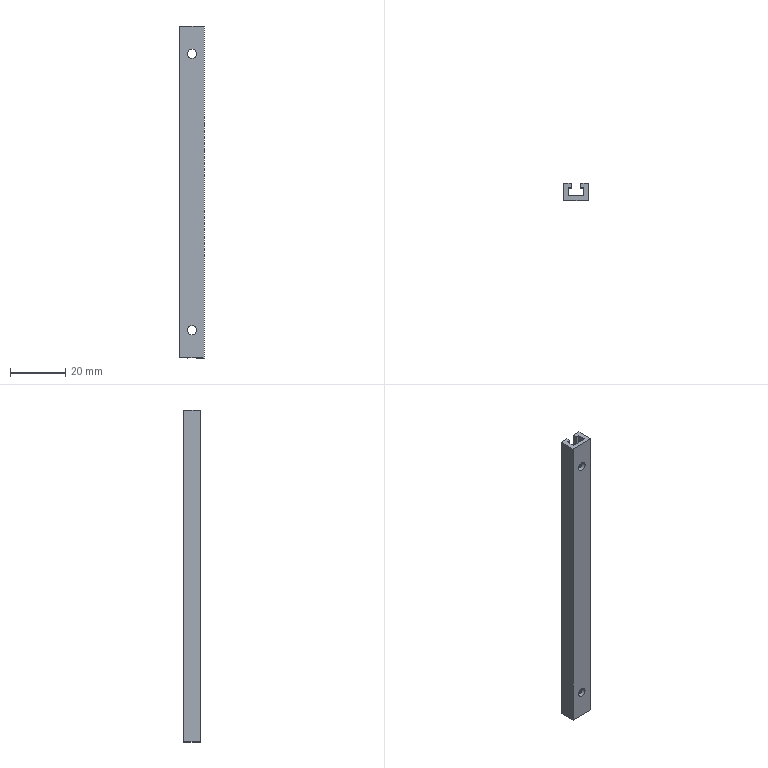Part | NX | 1 solid | 32 faces | box 9 x 6 x 120 mm | volume 3761 mm3 | plane 26 | cylinder 6 | commonest cylinder face diameters 6 x4 3.3 x2
STEP:
#1=CARTESIAN_POINT('',(6.2,-1.5,120.));
#2=VERTEX_POINT('',#1);
#3=CARTESIAN_POINT('',(6.2,-1.5,112.472));
#4=VERTEX_POINT('',#3);
#5=CARTESIAN_POINT('',(6.2,-1.5,120.));
#6=DIRECTION('',(0.,0.,-1.));
#7=VECTOR('',#6,1000.);
#8=LINE('',#5,#7);
#9=EDGE_CURVE('',#2,#4,#8,.T.);
#10=ORIENTED_EDGE('',*,*,#9,.T.);
#11=CARTESIAN_POINT('',(7.35,-1.5,110.937));
#12=VERTEX_POINT('',#11);
#13=CARTESIAN_POINT('',(4.5,-1.5,110.));
#14=DIRECTION('',(0.,1.,0.));
#15=DIRECTION('',(0.,0.,1.));
#16=AXIS2_PLACEMENT_3D('',#13,#14,#15);
#17=CIRCLE('',#16,3.);
#18=EDGE_CURVE('',#4,#12,#17,.T.);
#19=ORIENTED_EDGE('',*,*,#18,.T.);
#20=CARTESIAN_POINT('',(7.35,-1.5,120.));
#21=VERTEX_POINT('',#20);
#22=CARTESIAN_POINT('',(7.35,-1.5,120.));
#23=DIRECTION('',(0.,0.,-1.));
#24=VECTOR('',#23,1000.);
#25=LINE('',#22,#24);
#26=EDGE_CURVE('',#21,#12,#25,.T.);
#27=ORIENTED_EDGE('',*,*,#26,.F.);
#28=CARTESIAN_POINT('',(6.2,-1.5,120.));
#29=DIRECTION('',(1.,0.,0.));
#30=VECTOR('',#29,1000.);
#31=LINE('',#28,#30);
#32=EDGE_CURVE('',#2,#21,#31,.T.);
#33=ORIENTED_EDGE('',*,*,#32,.F.);
#34=EDGE_LOOP('',(#10,#19,#27,#33));
#35=FACE_BOUND('',#34,.T.);
#36=CARTESIAN_POINT('',(6.2,-1.5,120.));
#37=DIRECTION('',(0.,1.,0.));
#38=DIRECTION('',(0.,0.,1.));
#39=AXIS2_PLACEMENT_3D('',#36,#37,#38);
#40=PLANE('',#39);
#41=ADVANCED_FACE('',(#35),#40,.F.);
#42=CARTESIAN_POINT('',(1.65,-4.5,120.));
#43=VERTEX_POINT('',#42);
#44=CARTESIAN_POINT('',(1.65,-4.5,110.937));
#45=VERTEX_POINT('',#44);
#46=CARTESIAN_POINT('',(1.65,-4.5,120.));
#47=DIRECTION('',(0.,0.,-1.));
#48=VECTOR('',#47,1000.);
#49=LINE('',#46,#48);
#50=EDGE_CURVE('',#43,#45,#49,.T.);
#51=ORIENTED_EDGE('',*,*,#50,.T.);
#52=CARTESIAN_POINT('',(1.65,-1.5,110.937));
#53=VERTEX_POINT('',#52);
#54=CARTESIAN_POINT('',(1.65,-4.5,110.937));
#55=DIRECTION('',(0.,1.,0.));
#56=VECTOR('',#55,1000.);
#57=LINE('',#54,#56);
#58=EDGE_CURVE('',#45,#53,#57,.T.);
#59=ORIENTED_EDGE('',*,*,#58,.T.);
#60=CARTESIAN_POINT('',(1.65,-1.5,120.));
#61=VERTEX_POINT('',#60);
#62=CARTESIAN_POINT('',(1.65,-1.5,120.));
#63=DIRECTION('',(0.,0.,-1.));
#64=VECTOR('',#63,1000.);
#65=LINE('',#62,#64);
#66=EDGE_CURVE('',#61,#53,#65,.T.);
#67=ORIENTED_EDGE('',*,*,#66,.F.);
#68=CARTESIAN_POINT('',(1.65,-4.5,120.));
#69=DIRECTION('',(0.,1.,0.));
#70=VECTOR('',#69,1000.);
#71=LINE('',#68,#70);
#72=EDGE_CURVE('',#43,#61,#71,.T.);
#73=ORIENTED_EDGE('',*,*,#72,.F.);
#74=EDGE_LOOP('',(#51,#59,#67,#73));
#75=FACE_BOUND('',#74,.T.);
#76=CARTESIAN_POINT('',(1.65,-4.5,120.));
#77=DIRECTION('',(-1.,0.,0.));
#78=DIRECTION('',(0.,0.,1.));
#79=AXIS2_PLACEMENT_3D('',#76,#77,#78);
#80=PLANE('',#79);
#81=ADVANCED_FACE('',(#75),#80,.F.);
#82=CARTESIAN_POINT('',(2.8,-1.5,120.));
#83=VERTEX_POINT('',#82);
#84=CARTESIAN_POINT('',(2.8,-1.5,112.472));
#85=VERTEX_POINT('',#84);
#86=CARTESIAN_POINT('',(2.8,-1.5,120.));
#87=DIRECTION('',(0.,0.,-1.));
#88=VECTOR('',#87,1000.);
#89=LINE('',#86,#88);
#90=EDGE_CURVE('',#83,#85,#89,.T.);
#91=ORIENTED_EDGE('',*,*,#90,.T.);
#92=CARTESIAN_POINT('',(2.8,0.,112.472));
#93=VERTEX_POINT('',#92);
#94=CARTESIAN_POINT('',(2.8,-4.5,112.472));
#95=DIRECTION('',(0.,1.,0.));
#96=VECTOR('',#95,1000.);
#97=LINE('',#94,#96);
#98=EDGE_CURVE('',#85,#93,#97,.T.);
#99=ORIENTED_EDGE('',*,*,#98,.T.);
#100=CARTESIAN_POINT('',(2.8,0.,120.));
#101=VERTEX_POINT('',#100);
#102=CARTESIAN_POINT('',(2.8,0.,120.));
#103=DIRECTION('',(0.,0.,-1.));
#104=VECTOR('',#103,1000.);
#105=LINE('',#102,#104);
#106=EDGE_CURVE('',#101,#93,#105,.T.);
#107=ORIENTED_EDGE('',*,*,#106,.F.);
#108=CARTESIAN_POINT('',(2.8,-1.5,120.));
#109=DIRECTION('',(0.,1.,0.));
#110=VECTOR('',#109,1000.);
#111=LINE('',#108,#110);
#112=EDGE_CURVE('',#83,#101,#111,.T.);
#113=ORIENTED_EDGE('',*,*,#112,.F.);
#114=EDGE_LOOP('',(#91,#99,#107,#113));
#115=FACE_BOUND('',#114,.T.);
#116=CARTESIAN_POINT('',(2.8,-1.5,120.));
#117=DIRECTION('',(-1.,0.,0.));
#118=DIRECTION('',(0.,0.,1.));
#119=AXIS2_PLACEMENT_3D('',#116,#117,#118);
#120=PLANE('',#119);
#121=ADVANCED_FACE('',(#115),#120,.F.);
#122=CARTESIAN_POINT('',(6.2,-1.5,107.528));
#123=VERTEX_POINT('',#122);
#124=CARTESIAN_POINT('',(6.2,-1.5,12.472));
#125=VERTEX_POINT('',#124);
#126=CARTESIAN_POINT('',(6.2,-1.5,120.));
#127=DIRECTION('',(0.,0.,-1.));
#128=VECTOR('',#127,1000.);
#129=LINE('',#126,#128);
#130=EDGE_CURVE('',#123,#125,#129,.T.);
#131=ORIENTED_EDGE('',*,*,#130,.F.);
#132=CARTESIAN_POINT('',(6.2,0.,107.528));
#133=VERTEX_POINT('',#132);
#134=CARTESIAN_POINT('',(6.2,-4.5,107.528));
#135=DIRECTION('',(0.,1.,0.));
#136=VECTOR('',#135,1000.);
#137=LINE('',#134,#136);
#138=EDGE_CURVE('',#123,#133,#137,.T.);
#139=ORIENTED_EDGE('',*,*,#138,.T.);
#140=CARTESIAN_POINT('',(6.2,0.,12.472));
#141=VERTEX_POINT('',#140);
#142=CARTESIAN_POINT('',(6.2,0.,120.));
#143=DIRECTION('',(0.,0.,-1.));
#144=VECTOR('',#143,1000.);
#145=LINE('',#142,#144);
#146=EDGE_CURVE('',#133,#141,#145,.T.);
#147=ORIENTED_EDGE('',*,*,#146,.T.);
#148=CARTESIAN_POINT('',(6.2,-4.5,12.472));
#149=DIRECTION('',(0.,1.,0.));
#150=VECTOR('',#149,1000.);
#151=LINE('',#148,#150);
#152=EDGE_CURVE('',#141,#125,#151,.F.);
#153=ORIENTED_EDGE('',*,*,#152,.T.);
#154=EDGE_LOOP('',(#131,#139,#147,#153));
#155=FACE_BOUND('',#154,.T.);
#156=CARTESIAN_POINT('',(6.2,0.,120.));
#157=DIRECTION('',(1.,0.,0.));
#158=DIRECTION('',(0.,0.,-1.));
#159=AXIS2_PLACEMENT_3D('',#156,#157,#158);
#160=PLANE('',#159);
#161=ADVANCED_FACE('',(#155),#160,.F.);
#162=CARTESIAN_POINT('',(7.35,-4.5,109.063));
#163=VERTEX_POINT('',#162);
#164=CARTESIAN_POINT('',(7.35,-4.5,10.937));
#165=VERTEX_POINT('',#164);
#166=CARTESIAN_POINT('',(7.35,-4.5,120.));
#167=DIRECTION('',(0.,0.,-1.));
#168=VECTOR('',#167,1000.);
#169=LINE('',#166,#168);
#170=EDGE_CURVE('',#163,#165,#169,.T.);
#171=ORIENTED_EDGE('',*,*,#170,.F.);
#172=CARTESIAN_POINT('',(7.35,-1.5,109.063));
#173=VERTEX_POINT('',#172);
#174=CARTESIAN_POINT('',(7.35,-4.5,109.063));
#175=DIRECTION('',(0.,1.,0.));
#176=VECTOR('',#175,1000.);
#177=LINE('',#174,#176);
#178=EDGE_CURVE('',#163,#173,#177,.T.);
#179=ORIENTED_EDGE('',*,*,#178,.T.);
#180=CARTESIAN_POINT('',(7.35,-1.5,10.937));
#181=VERTEX_POINT('',#180);
#182=CARTESIAN_POINT('',(7.35,-1.5,120.));
#183=DIRECTION('',(0.,0.,-1.));
#184=VECTOR('',#183,1000.);
#185=LINE('',#182,#184);
#186=EDGE_CURVE('',#173,#181,#185,.T.);
#187=ORIENTED_EDGE('',*,*,#186,.T.);
#188=CARTESIAN_POINT('',(7.35,-4.5,10.937));
#189=DIRECTION('',(0.,1.,0.));
#190=VECTOR('',#189,1000.);
#191=LINE('',#188,#190);
#192=EDGE_CURVE('',#181,#165,#191,.F.);
#193=ORIENTED_EDGE('',*,*,#192,.T.);
#194=EDGE_LOOP('',(#171,#179,#187,#193));
#195=FACE_BOUND('',#194,.T.);
#196=CARTESIAN_POINT('',(7.35,-1.5,120.));
#197=DIRECTION('',(1.,0.,0.));
#198=DIRECTION('',(0.,0.,-1.));
#199=AXIS2_PLACEMENT_3D('',#196,#197,#198);
#200=PLANE('',#199);
#201=ADVANCED_FACE('',(#195),#200,.F.);
#202=CARTESIAN_POINT('',(2.8,-1.5,107.528));
#203=VERTEX_POINT('',#202);
#204=CARTESIAN_POINT('',(2.8,-1.5,12.472));
#205=VERTEX_POINT('',#204);
#206=CARTESIAN_POINT('',(2.8,-1.5,120.));
#207=DIRECTION('',(0.,0.,-1.));
#208=VECTOR('',#207,1000.);
#209=LINE('',#206,#208);
#210=EDGE_CURVE('',#203,#205,#209,.T.);
#211=ORIENTED_EDGE('',*,*,#210,.F.);
#212=CARTESIAN_POINT('',(1.65,-1.5,109.063));
#213=VERTEX_POINT('',#212);
#214=CARTESIAN_POINT('',(4.5,-1.5,110.));
#215=DIRECTION('',(0.,1.,0.));
#216=DIRECTION('',(0.,0.,1.));
#217=AXIS2_PLACEMENT_3D('',#214,#215,#216);
#218=CIRCLE('',#217,3.);
#219=EDGE_CURVE('',#203,#213,#218,.T.);
#220=ORIENTED_EDGE('',*,*,#219,.T.);
#221=CARTESIAN_POINT('',(1.65,-1.5,10.937));
#222=VERTEX_POINT('',#221);
#223=CARTESIAN_POINT('',(1.65,-1.5,120.));
#224=DIRECTION('',(0.,0.,-1.));
#225=VECTOR('',#224,1000.);
#226=LINE('',#223,#225);
#227=EDGE_CURVE('',#213,#222,#226,.T.);
#228=ORIENTED_EDGE('',*,*,#227,.T.);
#229=CARTESIAN_POINT('',(4.5,-1.5,10.));
#230=DIRECTION('',(0.,1.,0.));
#231=DIRECTION('',(0.,0.,1.));
#232=AXIS2_PLACEMENT_3D('',#229,#230,#231);
#233=CIRCLE('',#232,3.);
#234=EDGE_CURVE('',#222,#205,#233,.T.);
#235=ORIENTED_EDGE('',*,*,#234,.T.);
#236=EDGE_LOOP('',(#211,#220,#228,#235));
#237=FACE_BOUND('',#236,.T.);
#238=CARTESIAN_POINT('',(1.65,-1.5,120.));
#239=DIRECTION('',(0.,1.,0.));
#240=DIRECTION('',(0.,0.,1.));
#241=AXIS2_PLACEMENT_3D('',#238,#239,#240);
#242=PLANE('',#241);
#243=ADVANCED_FACE('',(#237),#242,.F.);
#244=CARTESIAN_POINT('',(6.2,-1.5,7.528));
#245=VERTEX_POINT('',#244);
#246=CARTESIAN_POINT('',(6.2,-1.5,0.));
#247=VERTEX_POINT('',#246);
#248=CARTESIAN_POINT('',(6.2,-1.5,120.));
#249=DIRECTION('',(0.,0.,-1.));
#250=VECTOR('',#249,1000.);
#251=LINE('',#248,#250);
#252=EDGE_CURVE('',#245,#247,#251,.T.);
#253=ORIENTED_EDGE('',*,*,#252,.F.);
#254=CARTESIAN_POINT('',(6.2,0.,7.528));
#255=VERTEX_POINT('',#254);
#256=CARTESIAN_POINT('',(6.2,-4.5,7.528));
#257=DIRECTION('',(0.,1.,0.));
#258=VECTOR('',#257,1000.);
#259=LINE('',#256,#258);
#260=EDGE_CURVE('',#245,#255,#259,.T.);
#261=ORIENTED_EDGE('',*,*,#260,.T.);
#262=CARTESIAN_POINT('',(6.2,0.,0.));
#263=VERTEX_POINT('',#262);
#264=CARTESIAN_POINT('',(6.2,0.,120.));
#265=DIRECTION('',(0.,0.,-1.));
#266=VECTOR('',#265,1000.);
#267=LINE('',#264,#266);
#268=EDGE_CURVE('',#255,#263,#267,.T.);
#269=ORIENTED_EDGE('',*,*,#268,.T.);
#270=CARTESIAN_POINT('',(6.2,0.,0.));
#271=DIRECTION('',(0.,-1.,0.));
#272=VECTOR('',#271,1000.);
#273=LINE('',#270,#272);
#274=EDGE_CURVE('',#263,#247,#273,.T.);
#275=ORIENTED_EDGE('',*,*,#274,.T.);
#276=EDGE_LOOP('',(#253,#261,#269,#275));
#277=FACE_BOUND('',#276,.T.);
#278=CARTESIAN_POINT('',(6.2,0.,120.));
#279=DIRECTION('',(1.,0.,0.));
#280=DIRECTION('',(0.,0.,-1.));
#281=AXIS2_PLACEMENT_3D('',#278,#279,#280);
#282=PLANE('',#281);
#283=ADVANCED_FACE('',(#277),#282,.F.);
#284=ORIENTED_EDGE('',*,*,#186,.F.);
#285=CARTESIAN_POINT('',(4.5,-1.5,110.));
#286=DIRECTION('',(0.,1.,0.));
#287=DIRECTION('',(0.,0.,1.));
#288=AXIS2_PLACEMENT_3D('',#285,#286,#287);
#289=CIRCLE('',#288,3.);
#290=EDGE_CURVE('',#173,#123,#289,.T.);
#291=ORIENTED_EDGE('',*,*,#290,.T.);
#292=ORIENTED_EDGE('',*,*,#130,.T.);
#293=CARTESIAN_POINT('',(4.5,-1.5,10.));
#294=DIRECTION('',(0.,1.,0.));
#295=DIRECTION('',(0.,0.,1.));
#296=AXIS2_PLACEMENT_3D('',#293,#294,#295);
#297=CIRCLE('',#296,3.);
#298=EDGE_CURVE('',#125,#181,#297,.T.);
#299=ORIENTED_EDGE('',*,*,#298,.T.);
#300=EDGE_LOOP('',(#284,#291,#292,#299));
#301=FACE_BOUND('',#300,.T.);
#302=CARTESIAN_POINT('',(6.2,-1.5,120.));
#303=DIRECTION('',(0.,1.,0.));
#304=DIRECTION('',(0.,0.,1.));
#305=AXIS2_PLACEMENT_3D('',#302,#303,#304);
#306=PLANE('',#305);
#307=ADVANCED_FACE('',(#301),#306,.F.);
#308=CARTESIAN_POINT('',(7.35,-4.5,9.063));
#309=VERTEX_POINT('',#308);
#310=CARTESIAN_POINT('',(7.35,-4.5,0.));
#311=VERTEX_POINT('',#310);
#312=CARTESIAN_POINT('',(7.35,-4.5,120.));
#313=DIRECTION('',(0.,0.,-1.));
#314=VECTOR('',#313,1000.);
#315=LINE('',#312,#314);
#316=EDGE_CURVE('',#309,#311,#315,.T.);
#317=ORIENTED_EDGE('',*,*,#316,.F.);
#318=CARTESIAN_POINT('',(7.35,-1.5,9.063));
#319=VERTEX_POINT('',#318);
#320=CARTESIAN_POINT('',(7.35,-4.5,9.063));
#321=DIRECTION('',(0.,1.,0.));
#322=VECTOR('',#321,1000.);
#323=LINE('',#320,#322);
#324=EDGE_CURVE('',#309,#319,#323,.T.);
#325=ORIENTED_EDGE('',*,*,#324,.T.);
#326=CARTESIAN_POINT('',(7.35,-1.5,0.));
#327=VERTEX_POINT('',#326);
#328=CARTESIAN_POINT('',(7.35,-1.5,120.));
#329=DIRECTION('',(0.,0.,-1.));
#330=VECTOR('',#329,1000.);
#331=LINE('',#328,#330);
#332=EDGE_CURVE('',#319,#327,#331,.T.);
#333=ORIENTED_EDGE('',*,*,#332,.T.);
#334=CARTESIAN_POINT('',(7.35,-1.5,0.));
#335=DIRECTION('',(0.,-1.,0.));
#336=VECTOR('',#335,1000.);
#337=LINE('',#334,#336);
#338=EDGE_CURVE('',#327,#311,#337,.T.);
#339=ORIENTED_EDGE('',*,*,#338,.T.);
#340=EDGE_LOOP('',(#317,#325,#333,#339));
#341=FACE_BOUND('',#340,.T.);
#342=CARTESIAN_POINT('',(7.35,-1.5,120.));
#343=DIRECTION('',(1.,0.,0.));
#344=DIRECTION('',(0.,0.,-1.));
#345=AXIS2_PLACEMENT_3D('',#342,#343,#344);
#346=PLANE('',#345);
#347=ADVANCED_FACE('',(#341),#346,.F.);
#348=ORIENTED_EDGE('',*,*,#227,.F.);
#349=CARTESIAN_POINT('',(1.65,-4.5,109.063));
#350=VERTEX_POINT('',#349);
#351=CARTESIAN_POINT('',(1.65,-4.5,109.063));
#352=DIRECTION('',(0.,1.,0.));
#353=VECTOR('',#352,1000.);
#354=LINE('',#351,#353);
#355=EDGE_CURVE('',#213,#350,#354,.F.);
#356=ORIENTED_EDGE('',*,*,#355,.T.);
#357=CARTESIAN_POINT('',(1.65,-4.5,10.937));
#358=VERTEX_POINT('',#357);
#359=CARTESIAN_POINT('',(1.65,-4.5,120.));
#360=DIRECTION('',(0.,0.,-1.));
#361=VECTOR('',#360,1000.);
#362=LINE('',#359,#361);
#363=EDGE_CURVE('',#350,#358,#362,.T.);
#364=ORIENTED_EDGE('',*,*,#363,.T.);
#365=CARTESIAN_POINT('',(1.65,-4.5,10.937));
#366=DIRECTION('',(0.,1.,0.));
#367=VECTOR('',#366,1000.);
#368=LINE('',#365,#367);
#369=EDGE_CURVE('',#358,#222,#368,.T.);
#370=ORIENTED_EDGE('',*,*,#369,.T.);
#371=EDGE_LOOP('',(#348,#356,#364,#370));
#372=FACE_BOUND('',#371,.T.);
#373=CARTESIAN_POINT('',(1.65,-4.5,120.));
#374=DIRECTION('',(-1.,0.,0.));
#375=DIRECTION('',(0.,0.,1.));
#376=AXIS2_PLACEMENT_3D('',#373,#374,#375);
#377=PLANE('',#376);
#378=ADVANCED_FACE('',(#372),#377,.F.);
#379=CARTESIAN_POINT('',(2.8,-1.5,7.528));
#380=VERTEX_POINT('',#379);
#381=CARTESIAN_POINT('',(2.8,-1.5,0.));
#382=VERTEX_POINT('',#381);
#383=CARTESIAN_POINT('',(2.8,-1.5,120.));
#384=DIRECTION('',(0.,0.,-1.));
#385=VECTOR('',#384,1000.);
#386=LINE('',#383,#385);
#387=EDGE_CURVE('',#380,#382,#386,.T.);
#388=ORIENTED_EDGE('',*,*,#387,.F.);
#389=CARTESIAN_POINT('',(1.65,-1.5,9.063));
#390=VERTEX_POINT('',#389);
#391=CARTESIAN_POINT('',(4.5,-1.5,10.));
#392=DIRECTION('',(0.,1.,0.));
#393=DIRECTION('',(0.,0.,1.));
#394=AXIS2_PLACEMENT_3D('',#391,#392,#393);
#395=CIRCLE('',#394,3.);
#396=EDGE_CURVE('',#380,#390,#395,.T.);
#397=ORIENTED_EDGE('',*,*,#396,.T.);
#398=CARTESIAN_POINT('',(1.65,-1.5,0.));
#399=VERTEX_POINT('',#398);
#400=CARTESIAN_POINT('',(1.65,-1.5,120.));
#401=DIRECTION('',(0.,0.,-1.));
#402=VECTOR('',#401,1000.);
#403=LINE('',#400,#402);
#404=EDGE_CURVE('',#390,#399,#403,.T.);
#405=ORIENTED_EDGE('',*,*,#404,.T.);
#406=CARTESIAN_POINT('',(1.65,-1.5,0.));
#407=DIRECTION('',(1.,0.,0.));
#408=VECTOR('',#407,1000.);
#409=LINE('',#406,#408);
#410=EDGE_CURVE('',#399,#382,#409,.T.);
#411=ORIENTED_EDGE('',*,*,#410,.T.);
#412=EDGE_LOOP('',(#388,#397,#405,#411));
#413=FACE_BOUND('',#412,.T.);
#414=CARTESIAN_POINT('',(1.65,-1.5,120.));
#415=DIRECTION('',(0.,1.,0.));
#416=DIRECTION('',(0.,0.,1.));
#417=AXIS2_PLACEMENT_3D('',#414,#415,#416);
#418=PLANE('',#417);
#419=ADVANCED_FACE('',(#413),#418,.F.);
#420=CARTESIAN_POINT('',(2.8,0.,107.528));
#421=VERTEX_POINT('',#420);
#422=CARTESIAN_POINT('',(2.8,0.,12.472));
#423=VERTEX_POINT('',#422);
#424=CARTESIAN_POINT('',(2.8,0.,120.));
#425=DIRECTION('',(0.,0.,-1.));
#426=VECTOR('',#425,1000.);
#427=LINE('',#424,#426);
#428=EDGE_CURVE('',#421,#423,#427,.T.);
#429=ORIENTED_EDGE('',*,*,#428,.F.);
#430=CARTESIAN_POINT('',(2.8,-4.5,107.528));
#431=DIRECTION('',(0.,1.,0.));
#432=VECTOR('',#431,1000.);
#433=LINE('',#430,#432);
#434=EDGE_CURVE('',#421,#203,#433,.F.);
#435=ORIENTED_EDGE('',*,*,#434,.T.);
#436=ORIENTED_EDGE('',*,*,#210,.T.);
#437=CARTESIAN_POINT('',(2.8,-4.5,12.472));
#438=DIRECTION('',(0.,1.,0.));
#439=VECTOR('',#438,1000.);
#440=LINE('',#437,#439);
#441=EDGE_CURVE('',#205,#423,#440,.T.);
#442=ORIENTED_EDGE('',*,*,#441,.T.);
#443=EDGE_LOOP('',(#429,#435,#436,#442));
#444=FACE_BOUND('',#443,.T.);
#445=CARTESIAN_POINT('',(2.8,-1.5,120.));
#446=DIRECTION('',(-1.,0.,0.));
#447=DIRECTION('',(0.,0.,1.));
#448=AXIS2_PLACEMENT_3D('',#445,#446,#447);
#449=PLANE('',#448);
#450=ADVANCED_FACE('',(#444),#449,.F.);
#451=ORIENTED_EDGE('',*,*,#106,.T.);
#452=CARTESIAN_POINT('',(4.5,0.,110.));
#453=DIRECTION('',(0.,1.,0.));
#454=DIRECTION('',(-1.,0.,0.));
#455=AXIS2_PLACEMENT_3D('',#452,#453,#454);
#456=CIRCLE('',#455,3.);
#457=EDGE_CURVE('',#421,#93,#456,.T.);
#458=ORIENTED_EDGE('',*,*,#457,.F.);
#459=ORIENTED_EDGE('',*,*,#428,.T.);
#460=CARTESIAN_POINT('',(2.8,0.,7.528));
#461=VERTEX_POINT('',#460);
#462=CARTESIAN_POINT('',(4.5,0.,10.));
#463=DIRECTION('',(0.,1.,0.));
#464=DIRECTION('',(-1.,0.,0.));
#465=AXIS2_PLACEMENT_3D('',#462,#463,#464);
#466=CIRCLE('',#465,3.);
#467=EDGE_CURVE('',#461,#423,#466,.T.);
#468=ORIENTED_EDGE('',*,*,#467,.F.);
#469=CARTESIAN_POINT('',(2.8,0.,0.));
#470=VERTEX_POINT('',#469);
#471=CARTESIAN_POINT('',(2.8,0.,120.));
#472=DIRECTION('',(0.,0.,-1.));
#473=VECTOR('',#472,1000.);
#474=LINE('',#471,#473);
#475=EDGE_CURVE('',#461,#470,#474,.T.);
#476=ORIENTED_EDGE('',*,*,#475,.T.);
#477=CARTESIAN_POINT('',(0.,0.,0.));
#478=VERTEX_POINT('',#477);
#479=CARTESIAN_POINT('',(2.8,0.,0.));
#480=DIRECTION('',(-1.,0.,0.));
#481=VECTOR('',#480,1000.);
#482=LINE('',#479,#481);
#483=EDGE_CURVE('',#470,#478,#482,.T.);
#484=ORIENTED_EDGE('',*,*,#483,.T.);
#485=CARTESIAN_POINT('',(0.,0.,120.));
#486=VERTEX_POINT('',#485);
#487=CARTESIAN_POINT('',(0.,0.,120.));
#488=DIRECTION('',(0.,0.,-1.));
#489=VECTOR('',#488,1000.);
#490=LINE('',#487,#489);
#491=EDGE_CURVE('',#486,#478,#490,.T.);
#492=ORIENTED_EDGE('',*,*,#491,.F.);
#493=CARTESIAN_POINT('',(2.8,0.,120.));
#494=DIRECTION('',(-1.,0.,0.));
#495=VECTOR('',#494,1000.);
#496=LINE('',#493,#495);
#497=EDGE_CURVE('',#101,#486,#496,.T.);
#498=ORIENTED_EDGE('',*,*,#497,.F.);
#499=EDGE_LOOP('',(#451,#458,#459,#468,#476,#484,#492,#498));
#500=FACE_BOUND('',#499,.T.);
#501=CARTESIAN_POINT('',(2.8,0.,120.));
#502=DIRECTION('',(0.,-1.,0.));
#503=DIRECTION('',(1.,0.,0.));
#504=AXIS2_PLACEMENT_3D('',#501,#502,#503);
#505=PLANE('',#504);
#506=ADVANCED_FACE('',(#500),#505,.F.);
#507=CARTESIAN_POINT('',(0.,-6.,0.));
#508=VERTEX_POINT('',#507);
#509=CARTESIAN_POINT('',(0.,0.,0.));
#510=DIRECTION('',(0.,-1.,0.));
#511=VECTOR('',#510,1000.);
#512=LINE('',#509,#511);
#513=EDGE_CURVE('',#478,#508,#512,.T.);
#514=ORIENTED_EDGE('',*,*,#513,.T.);
#515=CARTESIAN_POINT('',(0.,-6.,120.));
#516=VERTEX_POINT('',#515);
#517=CARTESIAN_POINT('',(0.,-6.,120.));
#518=DIRECTION('',(0.,0.,-1.));
#519=VECTOR('',#518,1000.);
#520=LINE('',#517,#519);
#521=EDGE_CURVE('',#516,#508,#520,.T.);
#522=ORIENTED_EDGE('',*,*,#521,.F.);
#523=CARTESIAN_POINT('',(0.,0.,120.));
#524=DIRECTION('',(0.,-1.,0.));
#525=VECTOR('',#524,1000.);
#526=LINE('',#523,#525);
#527=EDGE_CURVE('',#486,#516,#526,.T.);
#528=ORIENTED_EDGE('',*,*,#527,.F.);
#529=ORIENTED_EDGE('',*,*,#491,.T.);
#530=EDGE_LOOP('',(#514,#522,#528,#529));
#531=FACE_BOUND('',#530,.T.);
#532=CARTESIAN_POINT('',(0.,0.,120.));
#533=DIRECTION('',(1.,0.,0.));
#534=DIRECTION('',(0.,1.,0.));
#535=AXIS2_PLACEMENT_3D('',#532,#533,#534);
#536=PLANE('',#535);
#537=ADVANCED_FACE('',(#531),#536,.F.);
#538=CARTESIAN_POINT('',(4.5,-6.,11.65));
#539=VERTEX_POINT('',#538);
#540=CARTESIAN_POINT('',(4.5,-6.,10.));
#541=DIRECTION('',(0.,1.,0.));
#542=DIRECTION('',(0.,0.,1.));
#543=AXIS2_PLACEMENT_3D('',#540,#541,#542);
#544=CIRCLE('',#543,1.65);
#545=EDGE_CURVE('',#539,#539,#544,.T.);
#546=ORIENTED_EDGE('',*,*,#545,.T.);
#547=EDGE_LOOP('',(#546));
#548=FACE_BOUND('',#547,.T.);
#549=CARTESIAN_POINT('',(4.5,-6.,111.65));
#550=VERTEX_POINT('',#549);
#551=CARTESIAN_POINT('',(4.5,-6.,110.));
#552=DIRECTION('',(0.,1.,0.));
#553=DIRECTION('',(0.,0.,1.));
#554=AXIS2_PLACEMENT_3D('',#551,#552,#553);
#555=CIRCLE('',#554,1.65);
#556=EDGE_CURVE('',#550,#550,#555,.T.);
#557=ORIENTED_EDGE('',*,*,#556,.T.);
#558=EDGE_LOOP('',(#557));
#559=FACE_BOUND('',#558,.T.);
#560=CARTESIAN_POINT('',(9.,-6.,0.));
#561=VERTEX_POINT('',#560);
#562=CARTESIAN_POINT('',(0.,-6.,0.));
#563=DIRECTION('',(1.,0.,0.));
#564=VECTOR('',#563,1000.);
#565=LINE('',#562,#564);
#566=EDGE_CURVE('',#508,#561,#565,.T.);
#567=ORIENTED_EDGE('',*,*,#566,.T.);
#568=CARTESIAN_POINT('',(9.,-6.,120.));
#569=VERTEX_POINT('',#568);
#570=CARTESIAN_POINT('',(9.,-6.,120.));
#571=DIRECTION('',(0.,0.,-1.));
#572=VECTOR('',#571,1000.);
#573=LINE('',#570,#572);
#574=EDGE_CURVE('',#569,#561,#573,.T.);
#575=ORIENTED_EDGE('',*,*,#574,.F.);
#576=CARTESIAN_POINT('',(0.,-6.,120.));
#577=DIRECTION('',(1.,0.,0.));
#578=VECTOR('',#577,1000.);
#579=LINE('',#576,#578);
#580=EDGE_CURVE('',#516,#569,#579,.T.);
#581=ORIENTED_EDGE('',*,*,#580,.F.);
#582=ORIENTED_EDGE('',*,*,#521,.T.);
#583=EDGE_LOOP('',(#567,#575,#581,#582));
#584=FACE_BOUND('',#583,.T.);
#585=CARTESIAN_POINT('',(0.,-6.,120.));
#586=DIRECTION('',(0.,1.,0.));
#587=DIRECTION('',(0.,0.,1.));
#588=AXIS2_PLACEMENT_3D('',#585,#586,#587);
#589=PLANE('',#588);
#590=ADVANCED_FACE('',(#548,#559,#584),#589,.F.);
#591=CARTESIAN_POINT('',(9.,0.,0.));
#592=VERTEX_POINT('',#591);
#593=CARTESIAN_POINT('',(9.,-6.,0.));
#594=DIRECTION('',(0.,1.,0.));
#595=VECTOR('',#594,1000.);
#596=LINE('',#593,#595);
#597=EDGE_CURVE('',#561,#592,#596,.T.);
#598=ORIENTED_EDGE('',*,*,#597,.T.);
#599=CARTESIAN_POINT('',(9.,0.,120.));
#600=VERTEX_POINT('',#599);
#601=CARTESIAN_POINT('',(9.,0.,120.));
#602=DIRECTION('',(0.,0.,-1.));
#603=VECTOR('',#602,1000.);
#604=LINE('',#601,#603);
#605=EDGE_CURVE('',#600,#592,#604,.T.);
#606=ORIENTED_EDGE('',*,*,#605,.F.);
#607=CARTESIAN_POINT('',(9.,-6.,120.));
#608=DIRECTION('',(0.,1.,0.));
#609=VECTOR('',#608,1000.);
#610=LINE('',#607,#609);
#611=EDGE_CURVE('',#569,#600,#610,.T.);
#612=ORIENTED_EDGE('',*,*,#611,.F.);
#613=ORIENTED_EDGE('',*,*,#574,.T.);
#614=EDGE_LOOP('',(#598,#606,#612,#613));
#615=FACE_BOUND('',#614,.T.);
#616=CARTESIAN_POINT('',(9.,-6.,120.));
#617=DIRECTION('',(-1.,0.,0.));
#618=DIRECTION('',(0.,0.,1.));
#619=AXIS2_PLACEMENT_3D('',#616,#617,#618);
#620=PLANE('',#619);
#621=ADVANCED_FACE('',(#615),#620,.F.);
#622=ORIENTED_EDGE('',*,*,#146,.F.);
#623=CARTESIAN_POINT('',(6.2,0.,112.472));
#624=VERTEX_POINT('',#623);
#625=CARTESIAN_POINT('',(4.5,0.,110.));
#626=DIRECTION('',(0.,1.,0.));
#627=DIRECTION('',(-1.,0.,0.));
#628=AXIS2_PLACEMENT_3D('',#625,#626,#627);
#629=CIRCLE('',#628,3.);
#630=EDGE_CURVE('',#624,#133,#629,.T.);
#631=ORIENTED_EDGE('',*,*,#630,.F.);
#632=CARTESIAN_POINT('',(6.2,0.,120.));
#633=VERTEX_POINT('',#632);
#634=CARTESIAN_POINT('',(6.2,0.,120.));
#635=DIRECTION('',(0.,0.,-1.));
#636=VECTOR('',#635,1000.);
#637=LINE('',#634,#636);
#638=EDGE_CURVE('',#633,#624,#637,.T.);
#639=ORIENTED_EDGE('',*,*,#638,.F.);
#640=CARTESIAN_POINT('',(9.,0.,120.));
#641=DIRECTION('',(-1.,0.,0.));
#642=VECTOR('',#641,1000.);
#643=LINE('',#640,#642);
#644=EDGE_CURVE('',#600,#633,#643,.T.);
#645=ORIENTED_EDGE('',*,*,#644,.F.);
#646=ORIENTED_EDGE('',*,*,#605,.T.);
#647=CARTESIAN_POINT('',(9.,0.,0.));
#648=DIRECTION('',(-1.,0.,0.));
#649=VECTOR('',#648,1000.);
#650=LINE('',#647,#649);
#651=EDGE_CURVE('',#592,#263,#650,.T.);
#652=ORIENTED_EDGE('',*,*,#651,.T.);
#653=ORIENTED_EDGE('',*,*,#268,.F.);
#654=CARTESIAN_POINT('',(4.5,0.,10.));
#655=DIRECTION('',(0.,1.,0.));
#656=DIRECTION('',(-1.,0.,0.));
#657=AXIS2_PLACEMENT_3D('',#654,#655,#656);
#658=CIRCLE('',#657,3.);
#659=EDGE_CURVE('',#141,#255,#658,.T.);
#660=ORIENTED_EDGE('',*,*,#659,.F.);
#661=EDGE_LOOP('',(#622,#631,#639,#645,#646,#652,#653,#660));
#662=FACE_BOUND('',#661,.T.);
#663=CARTESIAN_POINT('',(9.,0.,120.));
#664=DIRECTION('',(0.,-1.,0.));
#665=DIRECTION('',(1.,0.,0.));
#666=AXIS2_PLACEMENT_3D('',#663,#664,#665);
#667=PLANE('',#666);
#668=ADVANCED_FACE('',(#662),#667,.F.);
#669=ORIENTED_EDGE('',*,*,#638,.T.);
#670=CARTESIAN_POINT('',(6.2,-4.5,112.472));
#671=DIRECTION('',(0.,1.,0.));
#672=VECTOR('',#671,1000.);
#673=LINE('',#670,#672);
#674=EDGE_CURVE('',#624,#4,#673,.F.);
#675=ORIENTED_EDGE('',*,*,#674,.T.);
#676=ORIENTED_EDGE('',*,*,#9,.F.);
#677=CARTESIAN_POINT('',(6.2,0.,120.));
#678=DIRECTION('',(0.,-1.,0.));
#679=VECTOR('',#678,1000.);
#680=LINE('',#677,#679);
#681=EDGE_CURVE('',#633,#2,#680,.T.);
#682=ORIENTED_EDGE('',*,*,#681,.F.);
#683=EDGE_LOOP('',(#669,#675,#676,#682));
#684=FACE_BOUND('',#683,.T.);
#685=CARTESIAN_POINT('',(6.2,0.,120.));
#686=DIRECTION('',(1.,0.,0.));
#687=DIRECTION('',(0.,0.,-1.));
#688=AXIS2_PLACEMENT_3D('',#685,#686,#687);
#689=PLANE('',#688);
#690=ADVANCED_FACE('',(#684),#689,.F.);
#691=ORIENTED_EDGE('',*,*,#332,.F.);
#692=CARTESIAN_POINT('',(4.5,-1.5,10.));
#693=DIRECTION('',(0.,1.,0.));
#694=DIRECTION('',(0.,0.,1.));
#695=AXIS2_PLACEMENT_3D('',#692,#693,#694);
#696=CIRCLE('',#695,3.);
#697=EDGE_CURVE('',#319,#245,#696,.T.);
#698=ORIENTED_EDGE('',*,*,#697,.T.);
#699=ORIENTED_EDGE('',*,*,#252,.T.);
#700=CARTESIAN_POINT('',(6.2,-1.5,0.));
#701=DIRECTION('',(1.,0.,0.));
#702=VECTOR('',#701,1000.);
#703=LINE('',#700,#702);
#704=EDGE_CURVE('',#247,#327,#703,.T.);
#705=ORIENTED_EDGE('',*,*,#704,.T.);
#706=EDGE_LOOP('',(#691,#698,#699,#705));
#707=FACE_BOUND('',#706,.T.);
#708=CARTESIAN_POINT('',(6.2,-1.5,120.));
#709=DIRECTION('',(0.,1.,0.));
#710=DIRECTION('',(0.,0.,1.));
#711=AXIS2_PLACEMENT_3D('',#708,#709,#710);
#712=PLANE('',#711);
#713=ADVANCED_FACE('',(#707),#712,.F.);
#714=ORIENTED_EDGE('',*,*,#26,.T.);
#715=CARTESIAN_POINT('',(7.35,-4.5,110.937));
#716=VERTEX_POINT('',#715);
#717=CARTESIAN_POINT('',(7.35,-4.5,110.937));
#718=DIRECTION('',(0.,1.,0.));
#719=VECTOR('',#718,1000.);
#720=LINE('',#717,#719);
#721=EDGE_CURVE('',#12,#716,#720,.F.);
#722=ORIENTED_EDGE('',*,*,#721,.T.);
#723=CARTESIAN_POINT('',(7.35,-4.5,120.));
#724=VERTEX_POINT('',#723);
#725=CARTESIAN_POINT('',(7.35,-4.5,120.));
#726=DIRECTION('',(0.,0.,-1.));
#727=VECTOR('',#726,1000.);
#728=LINE('',#725,#727);
#729=EDGE_CURVE('',#724,#716,#728,.T.);
#730=ORIENTED_EDGE('',*,*,#729,.F.);
#731=CARTESIAN_POINT('',(7.35,-1.5,120.));
#732=DIRECTION('',(0.,-1.,0.));
#733=VECTOR('',#732,1000.);
#734=LINE('',#731,#733);
#735=EDGE_CURVE('',#21,#724,#734,.T.);
#736=ORIENTED_EDGE('',*,*,#735,.F.);
#737=EDGE_LOOP('',(#714,#722,#730,#736));
#738=FACE_BOUND('',#737,.T.);
#739=CARTESIAN_POINT('',(7.35,-1.5,120.));
#740=DIRECTION('',(1.,0.,0.));
#741=DIRECTION('',(0.,0.,-1.));
#742=AXIS2_PLACEMENT_3D('',#739,#740,#741);
#743=PLANE('',#742);
#744=ADVANCED_FACE('',(#738),#743,.F.);
#745=ORIENTED_EDGE('',*,*,#363,.F.);
#746=CARTESIAN_POINT('',(4.5,-4.5,110.));
#747=DIRECTION('',(0.,1.,0.));
#748=DIRECTION('',(-1.,0.,0.));
#749=AXIS2_PLACEMENT_3D('',#746,#747,#748);
#750=CIRCLE('',#749,3.);
#751=EDGE_CURVE('',#350,#45,#750,.T.);
#752=ORIENTED_EDGE('',*,*,#751,.T.);
#753=ORIENTED_EDGE('',*,*,#50,.F.);
#754=CARTESIAN_POINT('',(7.35,-4.5,120.));
#755=DIRECTION('',(-1.,0.,0.));
#756=VECTOR('',#755,1000.);
#757=LINE('',#754,#756);
#758=EDGE_CURVE('',#724,#43,#757,.T.);
#759=ORIENTED_EDGE('',*,*,#758,.F.);
#760=ORIENTED_EDGE('',*,*,#729,.T.);
#761=CARTESIAN_POINT('',(4.5,-4.5,110.));
#762=DIRECTION('',(0.,1.,0.));
#763=DIRECTION('',(-1.,0.,0.));
#764=AXIS2_PLACEMENT_3D('',#761,#762,#763);
#765=CIRCLE('',#764,3.);
#766=EDGE_CURVE('',#716,#163,#765,.T.);
#767=ORIENTED_EDGE('',*,*,#766,.T.);
#768=ORIENTED_EDGE('',*,*,#170,.T.);
#769=CARTESIAN_POINT('',(4.5,-4.5,10.));
#770=DIRECTION('',(0.,1.,0.));
#771=DIRECTION('',(-1.,0.,0.));
#772=AXIS2_PLACEMENT_3D('',#769,#770,#771);
#773=CIRCLE('',#772,3.);
#774=EDGE_CURVE('',#165,#309,#773,.T.);
#775=ORIENTED_EDGE('',*,*,#774,.T.);
#776=ORIENTED_EDGE('',*,*,#316,.T.);
#777=CARTESIAN_POINT('',(1.65,-4.5,0.));
#778=VERTEX_POINT('',#777);
#779=CARTESIAN_POINT('',(7.35,-4.5,0.));
#780=DIRECTION('',(-1.,0.,0.));
#781=VECTOR('',#780,1000.);
#782=LINE('',#779,#781);
#783=EDGE_CURVE('',#311,#778,#782,.T.);
#784=ORIENTED_EDGE('',*,*,#783,.T.);
#785=CARTESIAN_POINT('',(1.65,-4.5,9.063));
#786=VERTEX_POINT('',#785);
#787=CARTESIAN_POINT('',(1.65,-4.5,120.));
#788=DIRECTION('',(0.,0.,-1.));
#789=VECTOR('',#788,1000.);
#790=LINE('',#787,#789);
#791=EDGE_CURVE('',#786,#778,#790,.T.);
#792=ORIENTED_EDGE('',*,*,#791,.F.);
#793=CARTESIAN_POINT('',(4.5,-4.5,10.));
#794=DIRECTION('',(0.,1.,0.));
#795=DIRECTION('',(-1.,0.,0.));
#796=AXIS2_PLACEMENT_3D('',#793,#794,#795);
#797=CIRCLE('',#796,3.);
#798=EDGE_CURVE('',#786,#358,#797,.T.);
#799=ORIENTED_EDGE('',*,*,#798,.T.);
#800=EDGE_LOOP('',(#745,#752,#753,#759,#760,#767,#768,#775,#776,#784,#792,#799));
#801=FACE_BOUND('',#800,.T.);
#802=CARTESIAN_POINT('',(4.5,-4.5,11.65));
#803=VERTEX_POINT('',#802);
#804=CARTESIAN_POINT('',(4.5,-4.5,10.));
#805=DIRECTION('',(0.,1.,0.));
#806=DIRECTION('',(0.,0.,1.));
#807=AXIS2_PLACEMENT_3D('',#804,#805,#806);
#808=CIRCLE('',#807,1.65);
#809=EDGE_CURVE('',#803,#803,#808,.T.);
#810=ORIENTED_EDGE('',*,*,#809,.F.);
#811=EDGE_LOOP('',(#810));
#812=FACE_BOUND('',#811,.T.);
#813=CARTESIAN_POINT('',(4.5,-4.5,111.65));
#814=VERTEX_POINT('',#813);
#815=CARTESIAN_POINT('',(4.5,-4.5,110.));
#816=DIRECTION('',(0.,1.,0.));
#817=DIRECTION('',(0.,0.,1.));
#818=AXIS2_PLACEMENT_3D('',#815,#816,#817);
#819=CIRCLE('',#818,1.65);
#820=EDGE_CURVE('',#814,#814,#819,.T.);
#821=ORIENTED_EDGE('',*,*,#820,.F.);
#822=EDGE_LOOP('',(#821));
#823=FACE_BOUND('',#822,.T.);
#824=CARTESIAN_POINT('',(7.35,-4.5,120.));
#825=DIRECTION('',(0.,-1.,0.));
#826=DIRECTION('',(1.,0.,0.));
#827=AXIS2_PLACEMENT_3D('',#824,#825,#826);
#828=PLANE('',#827);
#829=ADVANCED_FACE('',(#801,#812,#823),#828,.F.);
#830=ORIENTED_EDGE('',*,*,#404,.F.);
#831=CARTESIAN_POINT('',(1.65,-4.5,9.063));
#832=DIRECTION('',(0.,1.,0.));
#833=VECTOR('',#832,1000.);
#834=LINE('',#831,#833);
#835=EDGE_CURVE('',#390,#786,#834,.F.);
#836=ORIENTED_EDGE('',*,*,#835,.T.);
#837=ORIENTED_EDGE('',*,*,#791,.T.);
#838=CARTESIAN_POINT('',(1.65,-4.5,0.));
#839=DIRECTION('',(0.,1.,0.));
#840=VECTOR('',#839,1000.);
#841=LINE('',#838,#840);
#842=EDGE_CURVE('',#778,#399,#841,.T.);
#843=ORIENTED_EDGE('',*,*,#842,.T.);
#844=EDGE_LOOP('',(#830,#836,#837,#843));
#845=FACE_BOUND('',#844,.T.);
#846=CARTESIAN_POINT('',(1.65,-4.5,120.));
#847=DIRECTION('',(-1.,0.,0.));
#848=DIRECTION('',(0.,0.,1.));
#849=AXIS2_PLACEMENT_3D('',#846,#847,#848);
#850=PLANE('',#849);
#851=ADVANCED_FACE('',(#845),#850,.F.);
#852=ORIENTED_EDGE('',*,*,#66,.T.);
#853=CARTESIAN_POINT('',(4.5,-1.5,110.));
#854=DIRECTION('',(0.,1.,0.));
#855=DIRECTION('',(0.,0.,1.));
#856=AXIS2_PLACEMENT_3D('',#853,#854,#855);
#857=CIRCLE('',#856,3.);
#858=EDGE_CURVE('',#53,#85,#857,.T.);
#859=ORIENTED_EDGE('',*,*,#858,.T.);
#860=ORIENTED_EDGE('',*,*,#90,.F.);
#861=CARTESIAN_POINT('',(1.65,-1.5,120.));
#862=DIRECTION('',(1.,0.,0.));
#863=VECTOR('',#862,1000.);
#864=LINE('',#861,#863);
#865=EDGE_CURVE('',#61,#83,#864,.T.);
#866=ORIENTED_EDGE('',*,*,#865,.F.);
#867=EDGE_LOOP('',(#852,#859,#860,#866));
#868=FACE_BOUND('',#867,.T.);
#869=CARTESIAN_POINT('',(1.65,-1.5,120.));
#870=DIRECTION('',(0.,1.,0.));
#871=DIRECTION('',(0.,0.,1.));
#872=AXIS2_PLACEMENT_3D('',#869,#870,#871);
#873=PLANE('',#872);
#874=ADVANCED_FACE('',(#868),#873,.F.);
#875=ORIENTED_EDGE('',*,*,#475,.F.);
#876=CARTESIAN_POINT('',(2.8,-4.5,7.528));
#877=DIRECTION('',(0.,1.,0.));
#878=VECTOR('',#877,1000.);
#879=LINE('',#876,#878);
#880=EDGE_CURVE('',#461,#380,#879,.F.);
#881=ORIENTED_EDGE('',*,*,#880,.T.);
#882=ORIENTED_EDGE('',*,*,#387,.T.);
#883=CARTESIAN_POINT('',(2.8,-1.5,0.));
#884=DIRECTION('',(0.,1.,0.));
#885=VECTOR('',#884,1000.);
#886=LINE('',#883,#885);
#887=EDGE_CURVE('',#382,#470,#886,.T.);
#888=ORIENTED_EDGE('',*,*,#887,.T.);
#889=EDGE_LOOP('',(#875,#881,#882,#888));
#890=FACE_BOUND('',#889,.T.);
#891=CARTESIAN_POINT('',(2.8,-1.5,120.));
#892=DIRECTION('',(-1.,0.,0.));
#893=DIRECTION('',(0.,0.,1.));
#894=AXIS2_PLACEMENT_3D('',#891,#892,#893);
#895=PLANE('',#894);
#896=ADVANCED_FACE('',(#890),#895,.F.);
#897=ORIENTED_EDGE('',*,*,#497,.T.);
#898=ORIENTED_EDGE('',*,*,#527,.T.);
#899=ORIENTED_EDGE('',*,*,#580,.T.);
#900=ORIENTED_EDGE('',*,*,#611,.T.);
#901=ORIENTED_EDGE('',*,*,#644,.T.);
#902=ORIENTED_EDGE('',*,*,#681,.T.);
#903=ORIENTED_EDGE('',*,*,#32,.T.);
#904=ORIENTED_EDGE('',*,*,#735,.T.);
#905=ORIENTED_EDGE('',*,*,#758,.T.);
#906=ORIENTED_EDGE('',*,*,#72,.T.);
#907=ORIENTED_EDGE('',*,*,#865,.T.);
#908=ORIENTED_EDGE('',*,*,#112,.T.);
#909=EDGE_LOOP('',(#897,#898,#899,#900,#901,#902,#903,#904,#905,#906,#907,#908));
#910=FACE_BOUND('',#909,.T.);
#911=CARTESIAN_POINT('',(0.,0.,120.));
#912=DIRECTION('',(0.,0.,1.));
#913=DIRECTION('',(1.,0.,0.));
#914=AXIS2_PLACEMENT_3D('',#911,#912,#913);
#915=PLANE('',#914);
#916=ADVANCED_FACE('',(#910),#915,.T.);
#917=ORIENTED_EDGE('',*,*,#483,.F.);
#918=ORIENTED_EDGE('',*,*,#887,.F.);
#919=ORIENTED_EDGE('',*,*,#410,.F.);
#920=ORIENTED_EDGE('',*,*,#842,.F.);
#921=ORIENTED_EDGE('',*,*,#783,.F.);
#922=ORIENTED_EDGE('',*,*,#338,.F.);
#923=ORIENTED_EDGE('',*,*,#704,.F.);
#924=ORIENTED_EDGE('',*,*,#274,.F.);
#925=ORIENTED_EDGE('',*,*,#651,.F.);
#926=ORIENTED_EDGE('',*,*,#597,.F.);
#927=ORIENTED_EDGE('',*,*,#566,.F.);
#928=ORIENTED_EDGE('',*,*,#513,.F.);
#929=EDGE_LOOP('',(#917,#918,#919,#920,#921,#922,#923,#924,#925,#926,#927,#928));
#930=FACE_BOUND('',#929,.T.);
#931=CARTESIAN_POINT('',(0.,0.,0.));
#932=DIRECTION('',(0.,0.,1.));
#933=DIRECTION('',(1.,0.,0.));
#934=AXIS2_PLACEMENT_3D('',#931,#932,#933);
#935=PLANE('',#934);
#936=ADVANCED_FACE('',(#930),#935,.F.);
#937=ORIENTED_EDGE('',*,*,#556,.F.);
#938=EDGE_LOOP('',(#937));
#939=FACE_BOUND('',#938,.T.);
#940=ORIENTED_EDGE('',*,*,#820,.T.);
#941=EDGE_LOOP('',(#940));
#942=FACE_BOUND('',#941,.T.);
#943=CARTESIAN_POINT('',(4.5,-4.5,110.));
#944=DIRECTION('',(0.,1.,0.));
#945=DIRECTION('',(0.,0.,1.));
#946=AXIS2_PLACEMENT_3D('',#943,#944,#945);
#947=CYLINDRICAL_SURFACE('',#946,1.65);
#948=ADVANCED_FACE('',(#939,#942),#947,.F.);
#949=ORIENTED_EDGE('',*,*,#545,.F.);
#950=EDGE_LOOP('',(#949));
#951=FACE_BOUND('',#950,.T.);
#952=ORIENTED_EDGE('',*,*,#809,.T.);
#953=EDGE_LOOP('',(#952));
#954=FACE_BOUND('',#953,.T.);
#955=CARTESIAN_POINT('',(4.5,-4.5,10.));
#956=DIRECTION('',(0.,1.,0.));
#957=DIRECTION('',(0.,0.,1.));
#958=AXIS2_PLACEMENT_3D('',#955,#956,#957);
#959=CYLINDRICAL_SURFACE('',#958,1.65);
#960=ADVANCED_FACE('',(#951,#954),#959,.F.);
#961=ORIENTED_EDGE('',*,*,#798,.F.);
#962=ORIENTED_EDGE('',*,*,#835,.F.);
#963=ORIENTED_EDGE('',*,*,#396,.F.);
#964=ORIENTED_EDGE('',*,*,#880,.F.);
#965=ORIENTED_EDGE('',*,*,#467,.T.);
#966=ORIENTED_EDGE('',*,*,#441,.F.);
#967=ORIENTED_EDGE('',*,*,#234,.F.);
#968=ORIENTED_EDGE('',*,*,#369,.F.);
#969=EDGE_LOOP('',(#961,#962,#963,#964,#965,#966,#967,#968));
#970=FACE_BOUND('',#969,.T.);
#971=CARTESIAN_POINT('',(4.5,-4.5,10.));
#972=DIRECTION('',(0.,1.,0.));
#973=DIRECTION('',(-1.,0.,0.));
#974=AXIS2_PLACEMENT_3D('',#971,#972,#973);
#975=CYLINDRICAL_SURFACE('',#974,3.);
#976=ADVANCED_FACE('',(#970),#975,.F.);
#977=ORIENTED_EDGE('',*,*,#697,.F.);
#978=ORIENTED_EDGE('',*,*,#324,.F.);
#979=ORIENTED_EDGE('',*,*,#774,.F.);
#980=ORIENTED_EDGE('',*,*,#192,.F.);
#981=ORIENTED_EDGE('',*,*,#298,.F.);
#982=ORIENTED_EDGE('',*,*,#152,.F.);
#983=ORIENTED_EDGE('',*,*,#659,.T.);
#984=ORIENTED_EDGE('',*,*,#260,.F.);
#985=EDGE_LOOP('',(#977,#978,#979,#980,#981,#982,#983,#984));
#986=FACE_BOUND('',#985,.T.);
#987=CARTESIAN_POINT('',(4.5,-4.5,10.));
#988=DIRECTION('',(0.,1.,0.));
#989=DIRECTION('',(-1.,0.,0.));
#990=AXIS2_PLACEMENT_3D('',#987,#988,#989);
#991=CYLINDRICAL_SURFACE('',#990,3.);
#992=ADVANCED_FACE('',(#986),#991,.F.);
#993=ORIENTED_EDGE('',*,*,#219,.F.);
#994=ORIENTED_EDGE('',*,*,#434,.F.);
#995=ORIENTED_EDGE('',*,*,#457,.T.);
#996=ORIENTED_EDGE('',*,*,#98,.F.);
#997=ORIENTED_EDGE('',*,*,#858,.F.);
#998=ORIENTED_EDGE('',*,*,#58,.F.);
#999=ORIENTED_EDGE('',*,*,#751,.F.);
#1000=ORIENTED_EDGE('',*,*,#355,.F.);
#1001=EDGE_LOOP('',(#993,#994,#995,#996,#997,#998,#999,#1000));
#1002=FACE_BOUND('',#1001,.T.);
#1003=CARTESIAN_POINT('',(4.5,-4.5,110.));
#1004=DIRECTION('',(0.,1.,0.));
#1005=DIRECTION('',(-1.,0.,0.));
#1006=AXIS2_PLACEMENT_3D('',#1003,#1004,#1005);
#1007=CYLINDRICAL_SURFACE('',#1006,3.);
#1008=ADVANCED_FACE('',(#1002),#1007,.F.);
#1009=ORIENTED_EDGE('',*,*,#290,.F.);
#1010=ORIENTED_EDGE('',*,*,#178,.F.);
#1011=ORIENTED_EDGE('',*,*,#766,.F.);
#1012=ORIENTED_EDGE('',*,*,#721,.F.);
#1013=ORIENTED_EDGE('',*,*,#18,.F.);
#1014=ORIENTED_EDGE('',*,*,#674,.F.);
#1015=ORIENTED_EDGE('',*,*,#630,.T.);
#1016=ORIENTED_EDGE('',*,*,#138,.F.);
#1017=EDGE_LOOP('',(#1009,#1010,#1011,#1012,#1013,#1014,#1015,#1016));
#1018=FACE_BOUND('',#1017,.T.);
#1019=CARTESIAN_POINT('',(4.5,-4.5,110.));
#1020=DIRECTION('',(0.,1.,0.));
#1021=DIRECTION('',(-1.,0.,0.));
#1022=AXIS2_PLACEMENT_3D('',#1019,#1020,#1021);
#1023=CYLINDRICAL_SURFACE('',#1022,3.);
#1024=ADVANCED_FACE('',(#1018),#1023,.F.);
#1025=CLOSED_SHELL('',(#41,#81,#121,#161,#201,#243,#283,#307,#347,#378,#419,#450,#506,#537,#590,#621,#668,#690,#713,#744,#829,#851,#874,#896,#916,#936,#948,#960,#976,#992,#1008,#1024));
#1026=MANIFOLD_SOLID_BREP('',#1025);
#1027=(LENGTH_UNIT()NAMED_UNIT(*)SI_UNIT(.MILLI.,.METRE.));
#1028=UNCERTAINTY_MEASURE_WITH_UNIT(LENGTH_MEASURE(0.00001),#1027,'','');
#1029=(NAMED_UNIT(*)PLANE_ANGLE_UNIT()SI_UNIT($,.RADIAN.));
#1030=(NAMED_UNIT(*)SI_UNIT($,.STERADIAN.)SOLID_ANGLE_UNIT());
#1031=(GEOMETRIC_REPRESENTATION_CONTEXT(3)GLOBAL_UNCERTAINTY_ASSIGNED_CONTEXT((#1028))GLOBAL_UNIT_ASSIGNED_CONTEXT((#1027,#1029,#1030))REPRESENTATION_CONTEXT('',''));
#1032=ADVANCED_BREP_SHAPE_REPRESENTATION('',(#1026),#1031);